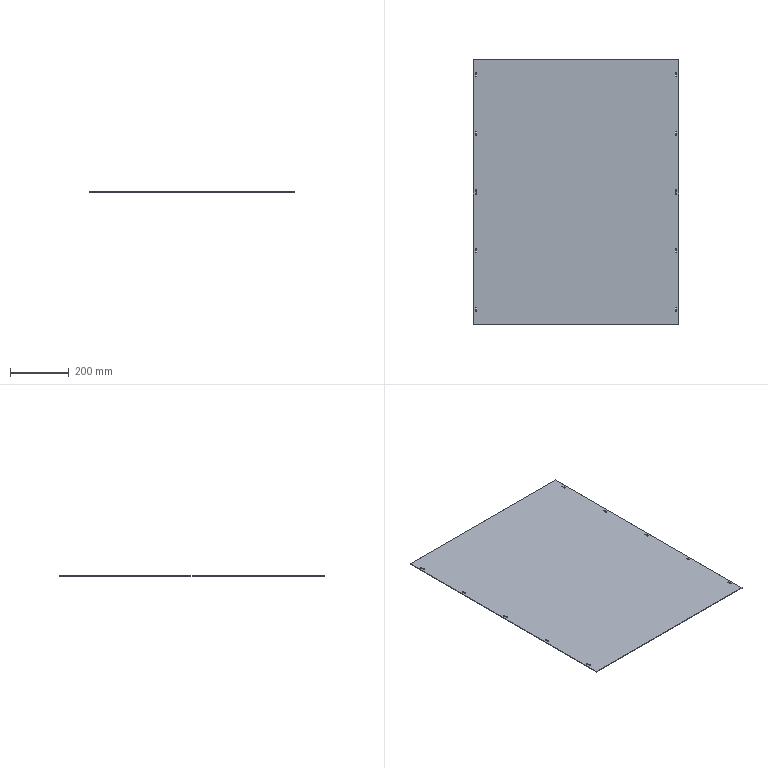Part | SolidWorks | features Extrusion 1, ICE 1 | 1 solid | 46 faces | box 700 x 900 x 2 mm | volume 1258782 mm3 | plane 26 | cylinder 20 | commonest cylinder face diameters 4.5 x20
STEP:
#1=CARTESIAN_POINT('',(350.,-450.,0.));
#2=VERTEX_POINT('',#1);
#3=CARTESIAN_POINT('',(350.,450.,0.));
#4=VERTEX_POINT('',#3);
#5=CARTESIAN_POINT('',(350.,450.,0.));
#6=DIRECTION('',(0.,1.,0.));
#7=VECTOR('',#6,1000.);
#8=LINE('',#5,#7);
#9=EDGE_CURVE('',#2,#4,#8,.T.);
#10=ORIENTED_EDGE('',*,*,#9,.T.);
#11=CARTESIAN_POINT('',(350.,450.,2.));
#12=VERTEX_POINT('',#11);
#13=CARTESIAN_POINT('',(350.,450.,2.));
#14=DIRECTION('',(0.,0.,-1.));
#15=VECTOR('',#14,1000.);
#16=LINE('',#13,#15);
#17=EDGE_CURVE('',#12,#4,#16,.T.);
#18=ORIENTED_EDGE('',*,*,#17,.F.);
#19=CARTESIAN_POINT('',(350.,-450.,2.));
#20=VERTEX_POINT('',#19);
#21=CARTESIAN_POINT('',(350.,450.,2.));
#22=DIRECTION('',(0.,1.,0.));
#23=VECTOR('',#22,1000.);
#24=LINE('',#21,#23);
#25=EDGE_CURVE('',#20,#12,#24,.T.);
#26=ORIENTED_EDGE('',*,*,#25,.F.);
#27=CARTESIAN_POINT('',(350.,-450.,2.));
#28=DIRECTION('',(0.,0.,-1.));
#29=VECTOR('',#28,1000.);
#30=LINE('',#27,#29);
#31=EDGE_CURVE('',#20,#2,#30,.T.);
#32=ORIENTED_EDGE('',*,*,#31,.T.);
#33=EDGE_LOOP('',(#10,#18,#26,#32));
#34=FACE_OUTER_BOUND('',#33,.T.);
#35=CARTESIAN_POINT('',(350.,450.,2.));
#36=DIRECTION('',(-1.,0.,0.));
#37=DIRECTION('',(0.,0.,1.));
#38=AXIS2_PLACEMENT_3D('',#35,#36,#37);
#39=PLANE('',#38);
#40=ADVANCED_FACE('',(#34),#39,.F.);
#41=CARTESIAN_POINT('',(-350.,450.,0.));
#42=VERTEX_POINT('',#41);
#43=CARTESIAN_POINT('',(-350.,450.,0.));
#44=DIRECTION('',(-1.,0.,0.));
#45=VECTOR('',#44,1000.);
#46=LINE('',#43,#45);
#47=EDGE_CURVE('',#4,#42,#46,.T.);
#48=ORIENTED_EDGE('',*,*,#47,.T.);
#49=CARTESIAN_POINT('',(-350.,450.,2.));
#50=VERTEX_POINT('',#49);
#51=CARTESIAN_POINT('',(-350.,450.,2.));
#52=DIRECTION('',(0.,0.,-1.));
#53=VECTOR('',#52,1000.);
#54=LINE('',#51,#53);
#55=EDGE_CURVE('',#50,#42,#54,.T.);
#56=ORIENTED_EDGE('',*,*,#55,.F.);
#57=CARTESIAN_POINT('',(-350.,450.,2.));
#58=DIRECTION('',(-1.,0.,0.));
#59=VECTOR('',#58,1000.);
#60=LINE('',#57,#59);
#61=EDGE_CURVE('',#12,#50,#60,.T.);
#62=ORIENTED_EDGE('',*,*,#61,.F.);
#63=ORIENTED_EDGE('',*,*,#17,.T.);
#64=EDGE_LOOP('',(#48,#56,#62,#63));
#65=FACE_OUTER_BOUND('',#64,.T.);
#66=CARTESIAN_POINT('',(-350.,450.,2.));
#67=DIRECTION('',(0.,-1.,0.));
#68=DIRECTION('',(0.,0.,-1.));
#69=AXIS2_PLACEMENT_3D('',#66,#67,#68);
#70=PLANE('',#69);
#71=ADVANCED_FACE('',(#65),#70,.F.);
#72=CARTESIAN_POINT('',(-350.,-450.,0.));
#73=VERTEX_POINT('',#72);
#74=CARTESIAN_POINT('',(-350.,450.,0.));
#75=DIRECTION('',(0.,-1.,0.));
#76=VECTOR('',#75,1000.);
#77=LINE('',#74,#76);
#78=EDGE_CURVE('',#42,#73,#77,.T.);
#79=ORIENTED_EDGE('',*,*,#78,.T.);
#80=CARTESIAN_POINT('',(-350.,-450.,2.));
#81=VERTEX_POINT('',#80);
#82=CARTESIAN_POINT('',(-350.,-450.,2.));
#83=DIRECTION('',(0.,0.,-1.));
#84=VECTOR('',#83,1000.);
#85=LINE('',#82,#84);
#86=EDGE_CURVE('',#81,#73,#85,.T.);
#87=ORIENTED_EDGE('',*,*,#86,.F.);
#88=CARTESIAN_POINT('',(-350.,450.,2.));
#89=DIRECTION('',(0.,-1.,0.));
#90=VECTOR('',#89,1000.);
#91=LINE('',#88,#90);
#92=EDGE_CURVE('',#50,#81,#91,.T.);
#93=ORIENTED_EDGE('',*,*,#92,.F.);
#94=ORIENTED_EDGE('',*,*,#55,.T.);
#95=EDGE_LOOP('',(#79,#87,#93,#94));
#96=FACE_OUTER_BOUND('',#95,.T.);
#97=CARTESIAN_POINT('',(-350.,450.,2.));
#98=DIRECTION('',(1.,0.,0.));
#99=DIRECTION('',(0.,0.,-1.));
#100=AXIS2_PLACEMENT_3D('',#97,#98,#99);
#101=PLANE('',#100);
#102=ADVANCED_FACE('',(#96),#101,.F.);
#103=CARTESIAN_POINT('',(-350.,-450.,0.));
#104=DIRECTION('',(1.,0.,0.));
#105=VECTOR('',#104,1000.);
#106=LINE('',#103,#105);
#107=EDGE_CURVE('',#73,#2,#106,.T.);
#108=ORIENTED_EDGE('',*,*,#107,.T.);
#109=ORIENTED_EDGE('',*,*,#31,.F.);
#110=CARTESIAN_POINT('',(-350.,-450.,2.));
#111=DIRECTION('',(1.,0.,0.));
#112=VECTOR('',#111,1000.);
#113=LINE('',#110,#112);
#114=EDGE_CURVE('',#81,#20,#113,.T.);
#115=ORIENTED_EDGE('',*,*,#114,.F.);
#116=ORIENTED_EDGE('',*,*,#86,.T.);
#117=EDGE_LOOP('',(#108,#109,#115,#116));
#118=FACE_OUTER_BOUND('',#117,.T.);
#119=CARTESIAN_POINT('',(-350.,-450.,2.));
#120=DIRECTION('',(0.,1.,0.));
#121=DIRECTION('',(0.,0.,1.));
#122=AXIS2_PLACEMENT_3D('',#119,#120,#121);
#123=PLANE('',#122);
#124=ADVANCED_FACE('',(#118),#123,.F.);
#125=CARTESIAN_POINT('',(337.75,-5.,2.));
#126=VERTEX_POINT('',#125);
#127=CARTESIAN_POINT('',(342.25,-5.,2.));
#128=VERTEX_POINT('',#127);
#129=CARTESIAN_POINT('',(340.,-5.,2.));
#130=DIRECTION('',(0.,0.,1.));
#131=DIRECTION('',(-1.,0.,0.));
#132=AXIS2_PLACEMENT_3D('',#129,#130,#131);
#133=CIRCLE('',#132,2.25);
#134=EDGE_CURVE('',#126,#128,#133,.T.);
#135=ORIENTED_EDGE('',*,*,#134,.F.);
#136=CARTESIAN_POINT('',(337.75,5.,2.));
#137=VERTEX_POINT('',#136);
#138=CARTESIAN_POINT('',(337.75,-5.,2.));
#139=DIRECTION('',(0.,-1.,0.));
#140=VECTOR('',#139,1000.);
#141=LINE('',#138,#140);
#142=EDGE_CURVE('',#137,#126,#141,.T.);
#143=ORIENTED_EDGE('',*,*,#142,.F.);
#144=CARTESIAN_POINT('',(342.25,5.,2.));
#145=VERTEX_POINT('',#144);
#146=CARTESIAN_POINT('',(340.,5.,2.));
#147=DIRECTION('',(0.,0.,1.));
#148=DIRECTION('',(-1.,0.,0.));
#149=AXIS2_PLACEMENT_3D('',#146,#147,#148);
#150=CIRCLE('',#149,2.25);
#151=EDGE_CURVE('',#145,#137,#150,.T.);
#152=ORIENTED_EDGE('',*,*,#151,.F.);
#153=CARTESIAN_POINT('',(342.25,-5.,2.));
#154=DIRECTION('',(0.,1.,0.));
#155=VECTOR('',#154,1000.);
#156=LINE('',#153,#155);
#157=EDGE_CURVE('',#128,#145,#156,.T.);
#158=ORIENTED_EDGE('',*,*,#157,.F.);
#159=EDGE_LOOP('',(#135,#143,#152,#158));
#160=FACE_BOUND('',#159,.T.);
#161=CARTESIAN_POINT('',(342.25,-195.,2.));
#162=VERTEX_POINT('',#161);
#163=CARTESIAN_POINT('',(337.75,-195.,2.));
#164=VERTEX_POINT('',#163);
#165=CARTESIAN_POINT('',(340.,-195.,2.));
#166=DIRECTION('',(0.,0.,1.));
#167=DIRECTION('',(1.,0.,0.));
#168=AXIS2_PLACEMENT_3D('',#165,#166,#167);
#169=CIRCLE('',#168,2.25);
#170=EDGE_CURVE('',#162,#164,#169,.T.);
#171=ORIENTED_EDGE('',*,*,#170,.F.);
#172=CARTESIAN_POINT('',(342.25,-205.,2.));
#173=VERTEX_POINT('',#172);
#174=CARTESIAN_POINT('',(342.25,-195.,2.));
#175=DIRECTION('',(0.,1.,0.));
#176=VECTOR('',#175,1000.);
#177=LINE('',#174,#176);
#178=EDGE_CURVE('',#173,#162,#177,.T.);
#179=ORIENTED_EDGE('',*,*,#178,.F.);
#180=CARTESIAN_POINT('',(337.75,-205.,2.));
#181=VERTEX_POINT('',#180);
#182=CARTESIAN_POINT('',(340.,-205.,2.));
#183=DIRECTION('',(0.,0.,1.));
#184=DIRECTION('',(1.,0.,0.));
#185=AXIS2_PLACEMENT_3D('',#182,#183,#184);
#186=CIRCLE('',#185,2.25);
#187=EDGE_CURVE('',#181,#173,#186,.T.);
#188=ORIENTED_EDGE('',*,*,#187,.F.);
#189=CARTESIAN_POINT('',(337.75,-195.,2.));
#190=DIRECTION('',(0.,-1.,0.));
#191=VECTOR('',#190,1000.);
#192=LINE('',#189,#191);
#193=EDGE_CURVE('',#164,#181,#192,.T.);
#194=ORIENTED_EDGE('',*,*,#193,.F.);
#195=EDGE_LOOP('',(#171,#179,#188,#194));
#196=FACE_BOUND('',#195,.T.);
#197=CARTESIAN_POINT('',(342.25,405.,2.));
#198=VERTEX_POINT('',#197);
#199=CARTESIAN_POINT('',(337.75,405.,2.));
#200=VERTEX_POINT('',#199);
#201=CARTESIAN_POINT('',(340.,405.,2.));
#202=DIRECTION('',(0.,0.,1.));
#203=DIRECTION('',(-1.,0.,0.));
#204=AXIS2_PLACEMENT_3D('',#201,#202,#203);
#205=CIRCLE('',#204,2.25);
#206=EDGE_CURVE('',#198,#200,#205,.T.);
#207=ORIENTED_EDGE('',*,*,#206,.F.);
#208=CARTESIAN_POINT('',(342.25,395.,2.));
#209=VERTEX_POINT('',#208);
#210=CARTESIAN_POINT('',(342.25,405.,2.));
#211=DIRECTION('',(0.,1.,0.));
#212=VECTOR('',#211,1000.);
#213=LINE('',#210,#212);
#214=EDGE_CURVE('',#209,#198,#213,.T.);
#215=ORIENTED_EDGE('',*,*,#214,.F.);
#216=CARTESIAN_POINT('',(337.75,395.,2.));
#217=VERTEX_POINT('',#216);
#218=CARTESIAN_POINT('',(340.,395.,2.));
#219=DIRECTION('',(0.,0.,1.));
#220=DIRECTION('',(-1.,0.,0.));
#221=AXIS2_PLACEMENT_3D('',#218,#219,#220);
#222=CIRCLE('',#221,2.25);
#223=EDGE_CURVE('',#217,#209,#222,.T.);
#224=ORIENTED_EDGE('',*,*,#223,.F.);
#225=CARTESIAN_POINT('',(337.75,405.,2.));
#226=DIRECTION('',(0.,-1.,0.));
#227=VECTOR('',#226,1000.);
#228=LINE('',#225,#227);
#229=EDGE_CURVE('',#200,#217,#228,.T.);
#230=ORIENTED_EDGE('',*,*,#229,.F.);
#231=EDGE_LOOP('',(#207,#215,#224,#230));
#232=FACE_BOUND('',#231,.T.);
#233=CARTESIAN_POINT('',(-342.25,195.,2.));
#234=VERTEX_POINT('',#233);
#235=CARTESIAN_POINT('',(-337.75,195.,2.));
#236=VERTEX_POINT('',#235);
#237=CARTESIAN_POINT('',(-340.,195.,2.));
#238=DIRECTION('',(0.,0.,1.));
#239=DIRECTION('',(1.,0.,0.));
#240=AXIS2_PLACEMENT_3D('',#237,#238,#239);
#241=CIRCLE('',#240,2.25);
#242=EDGE_CURVE('',#234,#236,#241,.T.);
#243=ORIENTED_EDGE('',*,*,#242,.F.);
#244=CARTESIAN_POINT('',(-342.25,205.,2.));
#245=VERTEX_POINT('',#244);
#246=CARTESIAN_POINT('',(-342.25,195.,2.));
#247=DIRECTION('',(0.,-1.,0.));
#248=VECTOR('',#247,1000.);
#249=LINE('',#246,#248);
#250=EDGE_CURVE('',#245,#234,#249,.T.);
#251=ORIENTED_EDGE('',*,*,#250,.F.);
#252=CARTESIAN_POINT('',(-337.75,205.,2.));
#253=VERTEX_POINT('',#252);
#254=CARTESIAN_POINT('',(-340.,205.,2.));
#255=DIRECTION('',(0.,0.,1.));
#256=DIRECTION('',(1.,0.,0.));
#257=AXIS2_PLACEMENT_3D('',#254,#255,#256);
#258=CIRCLE('',#257,2.25);
#259=EDGE_CURVE('',#253,#245,#258,.T.);
#260=ORIENTED_EDGE('',*,*,#259,.F.);
#261=CARTESIAN_POINT('',(-337.75,195.,2.));
#262=DIRECTION('',(0.,1.,0.));
#263=VECTOR('',#262,1000.);
#264=LINE('',#261,#263);
#265=EDGE_CURVE('',#236,#253,#264,.T.);
#266=ORIENTED_EDGE('',*,*,#265,.F.);
#267=EDGE_LOOP('',(#243,#251,#260,#266));
#268=FACE_BOUND('',#267,.T.);
#269=CARTESIAN_POINT('',(-342.25,-5.,2.));
#270=VERTEX_POINT('',#269);
#271=CARTESIAN_POINT('',(-337.75,-5.,2.));
#272=VERTEX_POINT('',#271);
#273=CARTESIAN_POINT('',(-340.,-5.,2.));
#274=DIRECTION('',(0.,0.,1.));
#275=DIRECTION('',(1.,0.,0.));
#276=AXIS2_PLACEMENT_3D('',#273,#274,#275);
#277=CIRCLE('',#276,2.25);
#278=EDGE_CURVE('',#270,#272,#277,.T.);
#279=ORIENTED_EDGE('',*,*,#278,.F.);
#280=CARTESIAN_POINT('',(-342.25,5.,2.));
#281=VERTEX_POINT('',#280);
#282=CARTESIAN_POINT('',(-342.25,-5.,2.));
#283=DIRECTION('',(0.,-1.,0.));
#284=VECTOR('',#283,1000.);
#285=LINE('',#282,#284);
#286=EDGE_CURVE('',#281,#270,#285,.T.);
#287=ORIENTED_EDGE('',*,*,#286,.F.);
#288=CARTESIAN_POINT('',(-337.75,5.,2.));
#289=VERTEX_POINT('',#288);
#290=CARTESIAN_POINT('',(-340.,5.,2.));
#291=DIRECTION('',(0.,0.,1.));
#292=DIRECTION('',(1.,0.,0.));
#293=AXIS2_PLACEMENT_3D('',#290,#291,#292);
#294=CIRCLE('',#293,2.25);
#295=EDGE_CURVE('',#289,#281,#294,.T.);
#296=ORIENTED_EDGE('',*,*,#295,.F.);
#297=CARTESIAN_POINT('',(-337.75,-5.,2.));
#298=DIRECTION('',(0.,1.,0.));
#299=VECTOR('',#298,1000.);
#300=LINE('',#297,#299);
#301=EDGE_CURVE('',#272,#289,#300,.T.);
#302=ORIENTED_EDGE('',*,*,#301,.F.);
#303=EDGE_LOOP('',(#279,#287,#296,#302));
#304=FACE_BOUND('',#303,.T.);
#305=CARTESIAN_POINT('',(337.75,195.,2.));
#306=VERTEX_POINT('',#305);
#307=CARTESIAN_POINT('',(342.25,195.,2.));
#308=VERTEX_POINT('',#307);
#309=CARTESIAN_POINT('',(340.,195.,2.));
#310=DIRECTION('',(0.,0.,1.));
#311=DIRECTION('',(-1.,0.,0.));
#312=AXIS2_PLACEMENT_3D('',#309,#310,#311);
#313=CIRCLE('',#312,2.25);
#314=EDGE_CURVE('',#306,#308,#313,.T.);
#315=ORIENTED_EDGE('',*,*,#314,.F.);
#316=CARTESIAN_POINT('',(337.75,205.,2.));
#317=VERTEX_POINT('',#316);
#318=CARTESIAN_POINT('',(337.75,195.,2.));
#319=DIRECTION('',(0.,-1.,0.));
#320=VECTOR('',#319,1000.);
#321=LINE('',#318,#320);
#322=EDGE_CURVE('',#317,#306,#321,.T.);
#323=ORIENTED_EDGE('',*,*,#322,.F.);
#324=CARTESIAN_POINT('',(342.25,205.,2.));
#325=VERTEX_POINT('',#324);
#326=CARTESIAN_POINT('',(340.,205.,2.));
#327=DIRECTION('',(0.,0.,1.));
#328=DIRECTION('',(-1.,0.,0.));
#329=AXIS2_PLACEMENT_3D('',#326,#327,#328);
#330=CIRCLE('',#329,2.25);
#331=EDGE_CURVE('',#325,#317,#330,.T.);
#332=ORIENTED_EDGE('',*,*,#331,.F.);
#333=CARTESIAN_POINT('',(342.25,195.,2.));
#334=DIRECTION('',(0.,1.,0.));
#335=VECTOR('',#334,1000.);
#336=LINE('',#333,#335);
#337=EDGE_CURVE('',#308,#325,#336,.T.);
#338=ORIENTED_EDGE('',*,*,#337,.F.);
#339=EDGE_LOOP('',(#315,#323,#332,#338));
#340=FACE_BOUND('',#339,.T.);
#341=CARTESIAN_POINT('',(-342.25,-405.,2.));
#342=VERTEX_POINT('',#341);
#343=CARTESIAN_POINT('',(-337.75,-405.,2.));
#344=VERTEX_POINT('',#343);
#345=CARTESIAN_POINT('',(-340.,-405.,2.));
#346=DIRECTION('',(0.,0.,1.));
#347=DIRECTION('',(-1.,0.,0.));
#348=AXIS2_PLACEMENT_3D('',#345,#346,#347);
#349=CIRCLE('',#348,2.25);
#350=EDGE_CURVE('',#342,#344,#349,.T.);
#351=ORIENTED_EDGE('',*,*,#350,.F.);
#352=CARTESIAN_POINT('',(-342.25,-395.,2.));
#353=VERTEX_POINT('',#352);
#354=CARTESIAN_POINT('',(-342.25,-405.,2.));
#355=DIRECTION('',(0.,-1.,0.));
#356=VECTOR('',#355,1000.);
#357=LINE('',#354,#356);
#358=EDGE_CURVE('',#353,#342,#357,.T.);
#359=ORIENTED_EDGE('',*,*,#358,.F.);
#360=CARTESIAN_POINT('',(-337.75,-395.,2.));
#361=VERTEX_POINT('',#360);
#362=CARTESIAN_POINT('',(-340.,-395.,2.));
#363=DIRECTION('',(0.,0.,1.));
#364=DIRECTION('',(-1.,0.,0.));
#365=AXIS2_PLACEMENT_3D('',#362,#363,#364);
#366=CIRCLE('',#365,2.25);
#367=EDGE_CURVE('',#361,#353,#366,.T.);
#368=ORIENTED_EDGE('',*,*,#367,.F.);
#369=CARTESIAN_POINT('',(-337.75,-405.,2.));
#370=DIRECTION('',(0.,1.,0.));
#371=VECTOR('',#370,1000.);
#372=LINE('',#369,#371);
#373=EDGE_CURVE('',#344,#361,#372,.T.);
#374=ORIENTED_EDGE('',*,*,#373,.F.);
#375=EDGE_LOOP('',(#351,#359,#368,#374));
#376=FACE_BOUND('',#375,.T.);
#377=CARTESIAN_POINT('',(337.75,-405.,2.));
#378=VERTEX_POINT('',#377);
#379=CARTESIAN_POINT('',(342.25,-405.,2.));
#380=VERTEX_POINT('',#379);
#381=CARTESIAN_POINT('',(340.,-405.,2.));
#382=DIRECTION('',(0.,0.,1.));
#383=DIRECTION('',(1.,0.,0.));
#384=AXIS2_PLACEMENT_3D('',#381,#382,#383);
#385=CIRCLE('',#384,2.25);
#386=EDGE_CURVE('',#378,#380,#385,.T.);
#387=ORIENTED_EDGE('',*,*,#386,.F.);
#388=CARTESIAN_POINT('',(337.75,-395.,2.));
#389=VERTEX_POINT('',#388);
#390=CARTESIAN_POINT('',(337.75,-405.,2.));
#391=DIRECTION('',(0.,-1.,0.));
#392=VECTOR('',#391,1000.);
#393=LINE('',#390,#392);
#394=EDGE_CURVE('',#389,#378,#393,.T.);
#395=ORIENTED_EDGE('',*,*,#394,.F.);
#396=CARTESIAN_POINT('',(342.25,-395.,2.));
#397=VERTEX_POINT('',#396);
#398=CARTESIAN_POINT('',(340.,-395.,2.));
#399=DIRECTION('',(0.,0.,1.));
#400=DIRECTION('',(1.,0.,0.));
#401=AXIS2_PLACEMENT_3D('',#398,#399,#400);
#402=CIRCLE('',#401,2.25);
#403=EDGE_CURVE('',#397,#389,#402,.T.);
#404=ORIENTED_EDGE('',*,*,#403,.F.);
#405=CARTESIAN_POINT('',(342.25,-405.,2.));
#406=DIRECTION('',(0.,1.,0.));
#407=VECTOR('',#406,1000.);
#408=LINE('',#405,#407);
#409=EDGE_CURVE('',#380,#397,#408,.T.);
#410=ORIENTED_EDGE('',*,*,#409,.F.);
#411=EDGE_LOOP('',(#387,#395,#404,#410));
#412=FACE_BOUND('',#411,.T.);
#413=CARTESIAN_POINT('',(-337.75,-195.,2.));
#414=VERTEX_POINT('',#413);
#415=CARTESIAN_POINT('',(-342.25,-195.,2.));
#416=VERTEX_POINT('',#415);
#417=CARTESIAN_POINT('',(-340.,-195.,2.));
#418=DIRECTION('',(0.,0.,1.));
#419=DIRECTION('',(-1.,0.,0.));
#420=AXIS2_PLACEMENT_3D('',#417,#418,#419);
#421=CIRCLE('',#420,2.25);
#422=EDGE_CURVE('',#414,#416,#421,.T.);
#423=ORIENTED_EDGE('',*,*,#422,.F.);
#424=CARTESIAN_POINT('',(-337.75,-205.,2.));
#425=VERTEX_POINT('',#424);
#426=CARTESIAN_POINT('',(-337.75,-195.,2.));
#427=DIRECTION('',(0.,1.,0.));
#428=VECTOR('',#427,1000.);
#429=LINE('',#426,#428);
#430=EDGE_CURVE('',#425,#414,#429,.T.);
#431=ORIENTED_EDGE('',*,*,#430,.F.);
#432=CARTESIAN_POINT('',(-342.25,-205.,2.));
#433=VERTEX_POINT('',#432);
#434=CARTESIAN_POINT('',(-340.,-205.,2.));
#435=DIRECTION('',(0.,0.,1.));
#436=DIRECTION('',(-1.,0.,0.));
#437=AXIS2_PLACEMENT_3D('',#434,#435,#436);
#438=CIRCLE('',#437,2.25);
#439=EDGE_CURVE('',#433,#425,#438,.T.);
#440=ORIENTED_EDGE('',*,*,#439,.F.);
#441=CARTESIAN_POINT('',(-342.25,-195.,2.));
#442=DIRECTION('',(0.,-1.,0.));
#443=VECTOR('',#442,1000.);
#444=LINE('',#441,#443);
#445=EDGE_CURVE('',#416,#433,#444,.T.);
#446=ORIENTED_EDGE('',*,*,#445,.F.);
#447=EDGE_LOOP('',(#423,#431,#440,#446));
#448=FACE_BOUND('',#447,.T.);
#449=CARTESIAN_POINT('',(-337.75,405.,2.));
#450=VERTEX_POINT('',#449);
#451=CARTESIAN_POINT('',(-342.25,405.,2.));
#452=VERTEX_POINT('',#451);
#453=CARTESIAN_POINT('',(-340.,405.,2.));
#454=DIRECTION('',(0.,0.,1.));
#455=DIRECTION('',(1.,0.,0.));
#456=AXIS2_PLACEMENT_3D('',#453,#454,#455);
#457=CIRCLE('',#456,2.25);
#458=EDGE_CURVE('',#450,#452,#457,.T.);
#459=ORIENTED_EDGE('',*,*,#458,.F.);
#460=CARTESIAN_POINT('',(-337.75,395.,2.));
#461=VERTEX_POINT('',#460);
#462=CARTESIAN_POINT('',(-337.75,405.,2.));
#463=DIRECTION('',(0.,1.,0.));
#464=VECTOR('',#463,1000.);
#465=LINE('',#462,#464);
#466=EDGE_CURVE('',#461,#450,#465,.T.);
#467=ORIENTED_EDGE('',*,*,#466,.F.);
#468=CARTESIAN_POINT('',(-342.25,395.,2.));
#469=VERTEX_POINT('',#468);
#470=CARTESIAN_POINT('',(-340.,395.,2.));
#471=DIRECTION('',(0.,0.,1.));
#472=DIRECTION('',(1.,0.,0.));
#473=AXIS2_PLACEMENT_3D('',#470,#471,#472);
#474=CIRCLE('',#473,2.25);
#475=EDGE_CURVE('',#469,#461,#474,.T.);
#476=ORIENTED_EDGE('',*,*,#475,.F.);
#477=CARTESIAN_POINT('',(-342.25,405.,2.));
#478=DIRECTION('',(0.,-1.,0.));
#479=VECTOR('',#478,1000.);
#480=LINE('',#477,#479);
#481=EDGE_CURVE('',#452,#469,#480,.T.);
#482=ORIENTED_EDGE('',*,*,#481,.F.);
#483=EDGE_LOOP('',(#459,#467,#476,#482));
#484=FACE_BOUND('',#483,.T.);
#485=ORIENTED_EDGE('',*,*,#25,.T.);
#486=ORIENTED_EDGE('',*,*,#61,.T.);
#487=ORIENTED_EDGE('',*,*,#92,.T.);
#488=ORIENTED_EDGE('',*,*,#114,.T.);
#489=EDGE_LOOP('',(#485,#486,#487,#488));
#490=FACE_OUTER_BOUND('',#489,.T.);
#491=CARTESIAN_POINT('',(0.,0.,2.));
#492=DIRECTION('',(0.,0.,1.));
#493=DIRECTION('',(1.,0.,0.));
#494=AXIS2_PLACEMENT_3D('',#491,#492,#493);
#495=PLANE('',#494);
#496=ADVANCED_FACE('',(#160,#196,#232,#268,#304,#340,#376,#412,#448,#484,#490),#495,.T.);
#497=CARTESIAN_POINT('',(337.75,5.,0.));
#498=VERTEX_POINT('',#497);
#499=CARTESIAN_POINT('',(337.75,-5.,0.));
#500=VERTEX_POINT('',#499);
#501=CARTESIAN_POINT('',(337.75,0.,0.));
#502=DIRECTION('',(0.,-1.,0.));
#503=VECTOR('',#502,1000.);
#504=LINE('',#501,#503);
#505=EDGE_CURVE('',#498,#500,#504,.T.);
#506=ORIENTED_EDGE('',*,*,#505,.T.);
#507=CARTESIAN_POINT('',(342.25,-5.,0.));
#508=VERTEX_POINT('',#507);
#509=CARTESIAN_POINT('',(340.,-5.,0.));
#510=DIRECTION('',(0.,0.,1.));
#511=DIRECTION('',(1.,0.,0.));
#512=AXIS2_PLACEMENT_3D('',#509,#510,#511);
#513=CIRCLE('',#512,2.25);
#514=EDGE_CURVE('',#500,#508,#513,.T.);
#515=ORIENTED_EDGE('',*,*,#514,.T.);
#516=CARTESIAN_POINT('',(342.25,5.,0.));
#517=VERTEX_POINT('',#516);
#518=CARTESIAN_POINT('',(342.25,0.,0.));
#519=DIRECTION('',(0.,1.,0.));
#520=VECTOR('',#519,1000.);
#521=LINE('',#518,#520);
#522=EDGE_CURVE('',#508,#517,#521,.T.);
#523=ORIENTED_EDGE('',*,*,#522,.T.);
#524=CARTESIAN_POINT('',(340.,5.,0.));
#525=DIRECTION('',(0.,0.,1.));
#526=DIRECTION('',(1.,0.,0.));
#527=AXIS2_PLACEMENT_3D('',#524,#525,#526);
#528=CIRCLE('',#527,2.25);
#529=EDGE_CURVE('',#517,#498,#528,.T.);
#530=ORIENTED_EDGE('',*,*,#529,.T.);
#531=EDGE_LOOP('',(#506,#515,#523,#530));
#532=FACE_BOUND('',#531,.T.);
#533=CARTESIAN_POINT('',(342.25,-205.,0.));
#534=VERTEX_POINT('',#533);
#535=CARTESIAN_POINT('',(342.25,-195.,0.));
#536=VERTEX_POINT('',#535);
#537=CARTESIAN_POINT('',(342.25,0.,0.));
#538=DIRECTION('',(0.,1.,0.));
#539=VECTOR('',#538,1000.);
#540=LINE('',#537,#539);
#541=EDGE_CURVE('',#534,#536,#540,.T.);
#542=ORIENTED_EDGE('',*,*,#541,.T.);
#543=CARTESIAN_POINT('',(337.75,-195.,0.));
#544=VERTEX_POINT('',#543);
#545=CARTESIAN_POINT('',(340.,-195.,0.));
#546=DIRECTION('',(0.,0.,1.));
#547=DIRECTION('',(1.,0.,0.));
#548=AXIS2_PLACEMENT_3D('',#545,#546,#547);
#549=CIRCLE('',#548,2.25);
#550=EDGE_CURVE('',#536,#544,#549,.T.);
#551=ORIENTED_EDGE('',*,*,#550,.T.);
#552=CARTESIAN_POINT('',(337.75,-205.,0.));
#553=VERTEX_POINT('',#552);
#554=CARTESIAN_POINT('',(337.75,0.,0.));
#555=DIRECTION('',(0.,-1.,0.));
#556=VECTOR('',#555,1000.);
#557=LINE('',#554,#556);
#558=EDGE_CURVE('',#544,#553,#557,.T.);
#559=ORIENTED_EDGE('',*,*,#558,.T.);
#560=CARTESIAN_POINT('',(340.,-205.,0.));
#561=DIRECTION('',(0.,0.,1.));
#562=DIRECTION('',(1.,0.,0.));
#563=AXIS2_PLACEMENT_3D('',#560,#561,#562);
#564=CIRCLE('',#563,2.25);
#565=EDGE_CURVE('',#553,#534,#564,.T.);
#566=ORIENTED_EDGE('',*,*,#565,.T.);
#567=EDGE_LOOP('',(#542,#551,#559,#566));
#568=FACE_BOUND('',#567,.T.);
#569=CARTESIAN_POINT('',(342.25,395.,0.));
#570=VERTEX_POINT('',#569);
#571=CARTESIAN_POINT('',(342.25,405.,0.));
#572=VERTEX_POINT('',#571);
#573=CARTESIAN_POINT('',(342.25,0.,0.));
#574=DIRECTION('',(0.,1.,0.));
#575=VECTOR('',#574,1000.);
#576=LINE('',#573,#575);
#577=EDGE_CURVE('',#570,#572,#576,.T.);
#578=ORIENTED_EDGE('',*,*,#577,.T.);
#579=CARTESIAN_POINT('',(337.75,405.,0.));
#580=VERTEX_POINT('',#579);
#581=CARTESIAN_POINT('',(340.,405.,0.));
#582=DIRECTION('',(0.,0.,1.));
#583=DIRECTION('',(1.,0.,0.));
#584=AXIS2_PLACEMENT_3D('',#581,#582,#583);
#585=CIRCLE('',#584,2.25);
#586=EDGE_CURVE('',#572,#580,#585,.T.);
#587=ORIENTED_EDGE('',*,*,#586,.T.);
#588=CARTESIAN_POINT('',(337.75,395.,0.));
#589=VERTEX_POINT('',#588);
#590=CARTESIAN_POINT('',(337.75,0.,0.));
#591=DIRECTION('',(0.,-1.,0.));
#592=VECTOR('',#591,1000.);
#593=LINE('',#590,#592);
#594=EDGE_CURVE('',#580,#589,#593,.T.);
#595=ORIENTED_EDGE('',*,*,#594,.T.);
#596=CARTESIAN_POINT('',(340.,395.,0.));
#597=DIRECTION('',(0.,0.,1.));
#598=DIRECTION('',(1.,0.,0.));
#599=AXIS2_PLACEMENT_3D('',#596,#597,#598);
#600=CIRCLE('',#599,2.25);
#601=EDGE_CURVE('',#589,#570,#600,.T.);
#602=ORIENTED_EDGE('',*,*,#601,.T.);
#603=EDGE_LOOP('',(#578,#587,#595,#602));
#604=FACE_BOUND('',#603,.T.);
#605=CARTESIAN_POINT('',(-342.25,205.,0.));
#606=VERTEX_POINT('',#605);
#607=CARTESIAN_POINT('',(-342.25,195.,0.));
#608=VERTEX_POINT('',#607);
#609=CARTESIAN_POINT('',(-342.25,0.,0.));
#610=DIRECTION('',(0.,-1.,0.));
#611=VECTOR('',#610,1000.);
#612=LINE('',#609,#611);
#613=EDGE_CURVE('',#606,#608,#612,.T.);
#614=ORIENTED_EDGE('',*,*,#613,.T.);
#615=CARTESIAN_POINT('',(-337.75,195.,0.));
#616=VERTEX_POINT('',#615);
#617=CARTESIAN_POINT('',(-340.,195.,0.));
#618=DIRECTION('',(0.,0.,1.));
#619=DIRECTION('',(1.,0.,0.));
#620=AXIS2_PLACEMENT_3D('',#617,#618,#619);
#621=CIRCLE('',#620,2.25);
#622=EDGE_CURVE('',#608,#616,#621,.T.);
#623=ORIENTED_EDGE('',*,*,#622,.T.);
#624=CARTESIAN_POINT('',(-337.75,205.,0.));
#625=VERTEX_POINT('',#624);
#626=CARTESIAN_POINT('',(-337.75,0.,0.));
#627=DIRECTION('',(0.,1.,0.));
#628=VECTOR('',#627,1000.);
#629=LINE('',#626,#628);
#630=EDGE_CURVE('',#616,#625,#629,.T.);
#631=ORIENTED_EDGE('',*,*,#630,.T.);
#632=CARTESIAN_POINT('',(-340.,205.,0.));
#633=DIRECTION('',(0.,0.,1.));
#634=DIRECTION('',(1.,0.,0.));
#635=AXIS2_PLACEMENT_3D('',#632,#633,#634);
#636=CIRCLE('',#635,2.25);
#637=EDGE_CURVE('',#625,#606,#636,.T.);
#638=ORIENTED_EDGE('',*,*,#637,.T.);
#639=EDGE_LOOP('',(#614,#623,#631,#638));
#640=FACE_BOUND('',#639,.T.);
#641=CARTESIAN_POINT('',(-342.25,5.,0.));
#642=VERTEX_POINT('',#641);
#643=CARTESIAN_POINT('',(-342.25,-5.,0.));
#644=VERTEX_POINT('',#643);
#645=CARTESIAN_POINT('',(-342.25,0.,0.));
#646=DIRECTION('',(0.,-1.,0.));
#647=VECTOR('',#646,1000.);
#648=LINE('',#645,#647);
#649=EDGE_CURVE('',#642,#644,#648,.T.);
#650=ORIENTED_EDGE('',*,*,#649,.T.);
#651=CARTESIAN_POINT('',(-337.75,-5.,0.));
#652=VERTEX_POINT('',#651);
#653=CARTESIAN_POINT('',(-340.,-5.,0.));
#654=DIRECTION('',(0.,0.,1.));
#655=DIRECTION('',(1.,0.,0.));
#656=AXIS2_PLACEMENT_3D('',#653,#654,#655);
#657=CIRCLE('',#656,2.25);
#658=EDGE_CURVE('',#644,#652,#657,.T.);
#659=ORIENTED_EDGE('',*,*,#658,.T.);
#660=CARTESIAN_POINT('',(-337.75,5.,0.));
#661=VERTEX_POINT('',#660);
#662=CARTESIAN_POINT('',(-337.75,0.,0.));
#663=DIRECTION('',(0.,1.,0.));
#664=VECTOR('',#663,1000.);
#665=LINE('',#662,#664);
#666=EDGE_CURVE('',#652,#661,#665,.T.);
#667=ORIENTED_EDGE('',*,*,#666,.T.);
#668=CARTESIAN_POINT('',(-340.,5.,0.));
#669=DIRECTION('',(0.,0.,1.));
#670=DIRECTION('',(1.,0.,0.));
#671=AXIS2_PLACEMENT_3D('',#668,#669,#670);
#672=CIRCLE('',#671,2.25);
#673=EDGE_CURVE('',#661,#642,#672,.T.);
#674=ORIENTED_EDGE('',*,*,#673,.T.);
#675=EDGE_LOOP('',(#650,#659,#667,#674));
#676=FACE_BOUND('',#675,.T.);
#677=CARTESIAN_POINT('',(337.75,205.,0.));
#678=VERTEX_POINT('',#677);
#679=CARTESIAN_POINT('',(337.75,195.,0.));
#680=VERTEX_POINT('',#679);
#681=CARTESIAN_POINT('',(337.75,0.,0.));
#682=DIRECTION('',(0.,-1.,0.));
#683=VECTOR('',#682,1000.);
#684=LINE('',#681,#683);
#685=EDGE_CURVE('',#678,#680,#684,.T.);
#686=ORIENTED_EDGE('',*,*,#685,.T.);
#687=CARTESIAN_POINT('',(342.25,195.,0.));
#688=VERTEX_POINT('',#687);
#689=CARTESIAN_POINT('',(340.,195.,0.));
#690=DIRECTION('',(0.,0.,1.));
#691=DIRECTION('',(1.,0.,0.));
#692=AXIS2_PLACEMENT_3D('',#689,#690,#691);
#693=CIRCLE('',#692,2.25);
#694=EDGE_CURVE('',#680,#688,#693,.T.);
#695=ORIENTED_EDGE('',*,*,#694,.T.);
#696=CARTESIAN_POINT('',(342.25,205.,0.));
#697=VERTEX_POINT('',#696);
#698=CARTESIAN_POINT('',(342.25,0.,0.));
#699=DIRECTION('',(0.,1.,0.));
#700=VECTOR('',#699,1000.);
#701=LINE('',#698,#700);
#702=EDGE_CURVE('',#688,#697,#701,.T.);
#703=ORIENTED_EDGE('',*,*,#702,.T.);
#704=CARTESIAN_POINT('',(340.,205.,0.));
#705=DIRECTION('',(0.,0.,1.));
#706=DIRECTION('',(1.,0.,0.));
#707=AXIS2_PLACEMENT_3D('',#704,#705,#706);
#708=CIRCLE('',#707,2.25);
#709=EDGE_CURVE('',#697,#678,#708,.T.);
#710=ORIENTED_EDGE('',*,*,#709,.T.);
#711=EDGE_LOOP('',(#686,#695,#703,#710));
#712=FACE_BOUND('',#711,.T.);
#713=CARTESIAN_POINT('',(-342.25,-395.,0.));
#714=VERTEX_POINT('',#713);
#715=CARTESIAN_POINT('',(-342.25,-405.,0.));
#716=VERTEX_POINT('',#715);
#717=CARTESIAN_POINT('',(-342.25,0.,0.));
#718=DIRECTION('',(0.,-1.,0.));
#719=VECTOR('',#718,1000.);
#720=LINE('',#717,#719);
#721=EDGE_CURVE('',#714,#716,#720,.T.);
#722=ORIENTED_EDGE('',*,*,#721,.T.);
#723=CARTESIAN_POINT('',(-337.75,-405.,0.));
#724=VERTEX_POINT('',#723);
#725=CARTESIAN_POINT('',(-340.,-405.,0.));
#726=DIRECTION('',(0.,0.,1.));
#727=DIRECTION('',(1.,0.,0.));
#728=AXIS2_PLACEMENT_3D('',#725,#726,#727);
#729=CIRCLE('',#728,2.25);
#730=EDGE_CURVE('',#716,#724,#729,.T.);
#731=ORIENTED_EDGE('',*,*,#730,.T.);
#732=CARTESIAN_POINT('',(-337.75,-395.,0.));
#733=VERTEX_POINT('',#732);
#734=CARTESIAN_POINT('',(-337.75,0.,0.));
#735=DIRECTION('',(0.,1.,0.));
#736=VECTOR('',#735,1000.);
#737=LINE('',#734,#736);
#738=EDGE_CURVE('',#724,#733,#737,.T.);
#739=ORIENTED_EDGE('',*,*,#738,.T.);
#740=CARTESIAN_POINT('',(-340.,-395.,0.));
#741=DIRECTION('',(0.,0.,1.));
#742=DIRECTION('',(1.,0.,0.));
#743=AXIS2_PLACEMENT_3D('',#740,#741,#742);
#744=CIRCLE('',#743,2.25);
#745=EDGE_CURVE('',#733,#714,#744,.T.);
#746=ORIENTED_EDGE('',*,*,#745,.T.);
#747=EDGE_LOOP('',(#722,#731,#739,#746));
#748=FACE_BOUND('',#747,.T.);
#749=CARTESIAN_POINT('',(337.75,-395.,0.));
#750=VERTEX_POINT('',#749);
#751=CARTESIAN_POINT('',(337.75,-405.,0.));
#752=VERTEX_POINT('',#751);
#753=CARTESIAN_POINT('',(337.75,0.,0.));
#754=DIRECTION('',(0.,-1.,0.));
#755=VECTOR('',#754,1000.);
#756=LINE('',#753,#755);
#757=EDGE_CURVE('',#750,#752,#756,.T.);
#758=ORIENTED_EDGE('',*,*,#757,.T.);
#759=CARTESIAN_POINT('',(342.25,-405.,0.));
#760=VERTEX_POINT('',#759);
#761=CARTESIAN_POINT('',(340.,-405.,0.));
#762=DIRECTION('',(0.,0.,1.));
#763=DIRECTION('',(1.,0.,0.));
#764=AXIS2_PLACEMENT_3D('',#761,#762,#763);
#765=CIRCLE('',#764,2.25);
#766=EDGE_CURVE('',#752,#760,#765,.T.);
#767=ORIENTED_EDGE('',*,*,#766,.T.);
#768=CARTESIAN_POINT('',(342.25,-395.,0.));
#769=VERTEX_POINT('',#768);
#770=CARTESIAN_POINT('',(342.25,0.,0.));
#771=DIRECTION('',(0.,1.,0.));
#772=VECTOR('',#771,1000.);
#773=LINE('',#770,#772);
#774=EDGE_CURVE('',#760,#769,#773,.T.);
#775=ORIENTED_EDGE('',*,*,#774,.T.);
#776=CARTESIAN_POINT('',(340.,-395.,0.));
#777=DIRECTION('',(0.,0.,1.));
#778=DIRECTION('',(1.,0.,0.));
#779=AXIS2_PLACEMENT_3D('',#776,#777,#778);
#780=CIRCLE('',#779,2.25);
#781=EDGE_CURVE('',#769,#750,#780,.T.);
#782=ORIENTED_EDGE('',*,*,#781,.T.);
#783=EDGE_LOOP('',(#758,#767,#775,#782));
#784=FACE_BOUND('',#783,.T.);
#785=CARTESIAN_POINT('',(-337.75,-205.,0.));
#786=VERTEX_POINT('',#785);
#787=CARTESIAN_POINT('',(-337.75,-195.,0.));
#788=VERTEX_POINT('',#787);
#789=CARTESIAN_POINT('',(-337.75,0.,0.));
#790=DIRECTION('',(0.,1.,0.));
#791=VECTOR('',#790,1000.);
#792=LINE('',#789,#791);
#793=EDGE_CURVE('',#786,#788,#792,.T.);
#794=ORIENTED_EDGE('',*,*,#793,.T.);
#795=CARTESIAN_POINT('',(-342.25,-195.,0.));
#796=VERTEX_POINT('',#795);
#797=CARTESIAN_POINT('',(-340.,-195.,0.));
#798=DIRECTION('',(0.,0.,1.));
#799=DIRECTION('',(1.,0.,0.));
#800=AXIS2_PLACEMENT_3D('',#797,#798,#799);
#801=CIRCLE('',#800,2.25);
#802=EDGE_CURVE('',#788,#796,#801,.T.);
#803=ORIENTED_EDGE('',*,*,#802,.T.);
#804=CARTESIAN_POINT('',(-342.25,-205.,0.));
#805=VERTEX_POINT('',#804);
#806=CARTESIAN_POINT('',(-342.25,0.,0.));
#807=DIRECTION('',(0.,-1.,0.));
#808=VECTOR('',#807,1000.);
#809=LINE('',#806,#808);
#810=EDGE_CURVE('',#796,#805,#809,.T.);
#811=ORIENTED_EDGE('',*,*,#810,.T.);
#812=CARTESIAN_POINT('',(-340.,-205.,0.));
#813=DIRECTION('',(0.,0.,1.));
#814=DIRECTION('',(1.,0.,0.));
#815=AXIS2_PLACEMENT_3D('',#812,#813,#814);
#816=CIRCLE('',#815,2.25);
#817=EDGE_CURVE('',#805,#786,#816,.T.);
#818=ORIENTED_EDGE('',*,*,#817,.T.);
#819=EDGE_LOOP('',(#794,#803,#811,#818));
#820=FACE_BOUND('',#819,.T.);
#821=CARTESIAN_POINT('',(-337.75,395.,0.));
#822=VERTEX_POINT('',#821);
#823=CARTESIAN_POINT('',(-337.75,405.,0.));
#824=VERTEX_POINT('',#823);
#825=CARTESIAN_POINT('',(-337.75,0.,0.));
#826=DIRECTION('',(0.,1.,0.));
#827=VECTOR('',#826,1000.);
#828=LINE('',#825,#827);
#829=EDGE_CURVE('',#822,#824,#828,.T.);
#830=ORIENTED_EDGE('',*,*,#829,.T.);
#831=CARTESIAN_POINT('',(-342.25,405.,0.));
#832=VERTEX_POINT('',#831);
#833=CARTESIAN_POINT('',(-340.,405.,0.));
#834=DIRECTION('',(0.,0.,1.));
#835=DIRECTION('',(1.,0.,0.));
#836=AXIS2_PLACEMENT_3D('',#833,#834,#835);
#837=CIRCLE('',#836,2.25);
#838=EDGE_CURVE('',#824,#832,#837,.T.);
#839=ORIENTED_EDGE('',*,*,#838,.T.);
#840=CARTESIAN_POINT('',(-342.25,395.,0.));
#841=VERTEX_POINT('',#840);
#842=CARTESIAN_POINT('',(-342.25,0.,0.));
#843=DIRECTION('',(0.,-1.,0.));
#844=VECTOR('',#843,1000.);
#845=LINE('',#842,#844);
#846=EDGE_CURVE('',#832,#841,#845,.T.);
#847=ORIENTED_EDGE('',*,*,#846,.T.);
#848=CARTESIAN_POINT('',(-340.,395.,0.));
#849=DIRECTION('',(0.,0.,1.));
#850=DIRECTION('',(1.,0.,0.));
#851=AXIS2_PLACEMENT_3D('',#848,#849,#850);
#852=CIRCLE('',#851,2.25);
#853=EDGE_CURVE('',#841,#822,#852,.T.);
#854=ORIENTED_EDGE('',*,*,#853,.T.);
#855=EDGE_LOOP('',(#830,#839,#847,#854));
#856=FACE_BOUND('',#855,.T.);
#857=ORIENTED_EDGE('',*,*,#9,.F.);
#858=ORIENTED_EDGE('',*,*,#107,.F.);
#859=ORIENTED_EDGE('',*,*,#78,.F.);
#860=ORIENTED_EDGE('',*,*,#47,.F.);
#861=EDGE_LOOP('',(#857,#858,#859,#860));
#862=FACE_OUTER_BOUND('',#861,.T.);
#863=CARTESIAN_POINT('',(0.,0.,0.));
#864=DIRECTION('',(0.,0.,1.));
#865=DIRECTION('',(1.,0.,0.));
#866=AXIS2_PLACEMENT_3D('',#863,#864,#865);
#867=PLANE('',#866);
#868=ADVANCED_FACE('',(#532,#568,#604,#640,#676,#712,#748,#784,#820,#856,#862),#867,.F.);
#869=CARTESIAN_POINT('',(-337.75,405.,-8.));
#870=DIRECTION('',(0.,0.,1.));
#871=VECTOR('',#870,1000.);
#872=LINE('',#869,#871);
#873=EDGE_CURVE('',#824,#450,#872,.T.);
#874=ORIENTED_EDGE('',*,*,#873,.T.);
#875=ORIENTED_EDGE('',*,*,#458,.T.);
#876=CARTESIAN_POINT('',(-342.25,405.,-8.));
#877=DIRECTION('',(0.,0.,1.));
#878=VECTOR('',#877,1000.);
#879=LINE('',#876,#878);
#880=EDGE_CURVE('',#832,#452,#879,.T.);
#881=ORIENTED_EDGE('',*,*,#880,.F.);
#882=ORIENTED_EDGE('',*,*,#838,.F.);
#883=EDGE_LOOP('',(#874,#875,#881,#882));
#884=FACE_OUTER_BOUND('',#883,.T.);
#885=CARTESIAN_POINT('',(-340.,405.,-8.));
#886=DIRECTION('',(0.,0.,1.));
#887=DIRECTION('',(1.,0.,0.));
#888=AXIS2_PLACEMENT_3D('',#885,#886,#887);
#889=CYLINDRICAL_SURFACE('',#888,2.25);
#890=ADVANCED_FACE('',(#884),#889,.F.);
#891=CARTESIAN_POINT('',(-337.75,395.,-8.));
#892=DIRECTION('',(0.,0.,1.));
#893=VECTOR('',#892,1000.);
#894=LINE('',#891,#893);
#895=EDGE_CURVE('',#822,#461,#894,.T.);
#896=ORIENTED_EDGE('',*,*,#895,.T.);
#897=ORIENTED_EDGE('',*,*,#466,.T.);
#898=ORIENTED_EDGE('',*,*,#873,.F.);
#899=ORIENTED_EDGE('',*,*,#829,.F.);
#900=EDGE_LOOP('',(#896,#897,#898,#899));
#901=FACE_OUTER_BOUND('',#900,.T.);
#902=CARTESIAN_POINT('',(-337.75,405.,-8.));
#903=DIRECTION('',(1.,0.,0.));
#904=DIRECTION('',(0.,0.,-1.));
#905=AXIS2_PLACEMENT_3D('',#902,#903,#904);
#906=PLANE('',#905);
#907=ADVANCED_FACE('',(#901),#906,.F.);
#908=CARTESIAN_POINT('',(-342.25,395.,-8.));
#909=DIRECTION('',(0.,0.,1.));
#910=VECTOR('',#909,1000.);
#911=LINE('',#908,#910);
#912=EDGE_CURVE('',#841,#469,#911,.T.);
#913=ORIENTED_EDGE('',*,*,#912,.T.);
#914=ORIENTED_EDGE('',*,*,#475,.T.);
#915=ORIENTED_EDGE('',*,*,#895,.F.);
#916=ORIENTED_EDGE('',*,*,#853,.F.);
#917=EDGE_LOOP('',(#913,#914,#915,#916));
#918=FACE_OUTER_BOUND('',#917,.T.);
#919=CARTESIAN_POINT('',(-340.,395.,-8.));
#920=DIRECTION('',(0.,0.,1.));
#921=DIRECTION('',(1.,0.,0.));
#922=AXIS2_PLACEMENT_3D('',#919,#920,#921);
#923=CYLINDRICAL_SURFACE('',#922,2.25);
#924=ADVANCED_FACE('',(#918),#923,.F.);
#925=ORIENTED_EDGE('',*,*,#880,.T.);
#926=ORIENTED_EDGE('',*,*,#481,.T.);
#927=ORIENTED_EDGE('',*,*,#912,.F.);
#928=ORIENTED_EDGE('',*,*,#846,.F.);
#929=EDGE_LOOP('',(#925,#926,#927,#928));
#930=FACE_OUTER_BOUND('',#929,.T.);
#931=CARTESIAN_POINT('',(-342.25,405.,-8.));
#932=DIRECTION('',(-1.,0.,0.));
#933=DIRECTION('',(0.,0.,1.));
#934=AXIS2_PLACEMENT_3D('',#931,#932,#933);
#935=PLANE('',#934);
#936=ADVANCED_FACE('',(#930),#935,.F.);
#937=CARTESIAN_POINT('',(-337.75,-195.,-8.));
#938=DIRECTION('',(0.,0.,1.));
#939=VECTOR('',#938,1000.);
#940=LINE('',#937,#939);
#941=EDGE_CURVE('',#788,#414,#940,.T.);
#942=ORIENTED_EDGE('',*,*,#941,.T.);
#943=ORIENTED_EDGE('',*,*,#422,.T.);
#944=CARTESIAN_POINT('',(-342.25,-195.,-8.));
#945=DIRECTION('',(0.,0.,1.));
#946=VECTOR('',#945,1000.);
#947=LINE('',#944,#946);
#948=EDGE_CURVE('',#796,#416,#947,.T.);
#949=ORIENTED_EDGE('',*,*,#948,.F.);
#950=ORIENTED_EDGE('',*,*,#802,.F.);
#951=EDGE_LOOP('',(#942,#943,#949,#950));
#952=FACE_OUTER_BOUND('',#951,.T.);
#953=CARTESIAN_POINT('',(-340.,-195.,-8.));
#954=DIRECTION('',(0.,0.,1.));
#955=DIRECTION('',(1.,0.,0.));
#956=AXIS2_PLACEMENT_3D('',#953,#954,#955);
#957=CYLINDRICAL_SURFACE('',#956,2.25);
#958=ADVANCED_FACE('',(#952),#957,.F.);
#959=CARTESIAN_POINT('',(-337.75,-205.,-8.));
#960=DIRECTION('',(0.,0.,1.));
#961=VECTOR('',#960,1000.);
#962=LINE('',#959,#961);
#963=EDGE_CURVE('',#786,#425,#962,.T.);
#964=ORIENTED_EDGE('',*,*,#963,.T.);
#965=ORIENTED_EDGE('',*,*,#430,.T.);
#966=ORIENTED_EDGE('',*,*,#941,.F.);
#967=ORIENTED_EDGE('',*,*,#793,.F.);
#968=EDGE_LOOP('',(#964,#965,#966,#967));
#969=FACE_OUTER_BOUND('',#968,.T.);
#970=CARTESIAN_POINT('',(-337.75,-195.,-8.));
#971=DIRECTION('',(1.,0.,0.));
#972=DIRECTION('',(0.,0.,-1.));
#973=AXIS2_PLACEMENT_3D('',#970,#971,#972);
#974=PLANE('',#973);
#975=ADVANCED_FACE('',(#969),#974,.F.);
#976=CARTESIAN_POINT('',(-342.25,-205.,-8.));
#977=DIRECTION('',(0.,0.,1.));
#978=VECTOR('',#977,1000.);
#979=LINE('',#976,#978);
#980=EDGE_CURVE('',#805,#433,#979,.T.);
#981=ORIENTED_EDGE('',*,*,#980,.T.);
#982=ORIENTED_EDGE('',*,*,#439,.T.);
#983=ORIENTED_EDGE('',*,*,#963,.F.);
#984=ORIENTED_EDGE('',*,*,#817,.F.);
#985=EDGE_LOOP('',(#981,#982,#983,#984));
#986=FACE_OUTER_BOUND('',#985,.T.);
#987=CARTESIAN_POINT('',(-340.,-205.,-8.));
#988=DIRECTION('',(0.,0.,1.));
#989=DIRECTION('',(1.,0.,0.));
#990=AXIS2_PLACEMENT_3D('',#987,#988,#989);
#991=CYLINDRICAL_SURFACE('',#990,2.25);
#992=ADVANCED_FACE('',(#986),#991,.F.);
#993=ORIENTED_EDGE('',*,*,#948,.T.);
#994=ORIENTED_EDGE('',*,*,#445,.T.);
#995=ORIENTED_EDGE('',*,*,#980,.F.);
#996=ORIENTED_EDGE('',*,*,#810,.F.);
#997=EDGE_LOOP('',(#993,#994,#995,#996));
#998=FACE_OUTER_BOUND('',#997,.T.);
#999=CARTESIAN_POINT('',(-342.25,-195.,-8.));
#1000=DIRECTION('',(-1.,0.,0.));
#1001=DIRECTION('',(0.,0.,1.));
#1002=AXIS2_PLACEMENT_3D('',#999,#1000,#1001);
#1003=PLANE('',#1002);
#1004=ADVANCED_FACE('',(#998),#1003,.F.);
#1005=CARTESIAN_POINT('',(337.75,-405.,-8.));
#1006=DIRECTION('',(0.,0.,1.));
#1007=VECTOR('',#1006,1000.);
#1008=LINE('',#1005,#1007);
#1009=EDGE_CURVE('',#752,#378,#1008,.T.);
#1010=ORIENTED_EDGE('',*,*,#1009,.T.);
#1011=ORIENTED_EDGE('',*,*,#386,.T.);
#1012=CARTESIAN_POINT('',(342.25,-405.,-8.));
#1013=DIRECTION('',(0.,0.,1.));
#1014=VECTOR('',#1013,1000.);
#1015=LINE('',#1012,#1014);
#1016=EDGE_CURVE('',#760,#380,#1015,.T.);
#1017=ORIENTED_EDGE('',*,*,#1016,.F.);
#1018=ORIENTED_EDGE('',*,*,#766,.F.);
#1019=EDGE_LOOP('',(#1010,#1011,#1017,#1018));
#1020=FACE_OUTER_BOUND('',#1019,.T.);
#1021=CARTESIAN_POINT('',(340.,-405.,-8.));
#1022=DIRECTION('',(0.,0.,1.));
#1023=DIRECTION('',(1.,0.,0.));
#1024=AXIS2_PLACEMENT_3D('',#1021,#1022,#1023);
#1025=CYLINDRICAL_SURFACE('',#1024,2.25);
#1026=ADVANCED_FACE('',(#1020),#1025,.F.);
#1027=CARTESIAN_POINT('',(337.75,-395.,-8.));
#1028=DIRECTION('',(0.,0.,1.));
#1029=VECTOR('',#1028,1000.);
#1030=LINE('',#1027,#1029);
#1031=EDGE_CURVE('',#750,#389,#1030,.T.);
#1032=ORIENTED_EDGE('',*,*,#1031,.T.);
#1033=ORIENTED_EDGE('',*,*,#394,.T.);
#1034=ORIENTED_EDGE('',*,*,#1009,.F.);
#1035=ORIENTED_EDGE('',*,*,#757,.F.);
#1036=EDGE_LOOP('',(#1032,#1033,#1034,#1035));
#1037=FACE_OUTER_BOUND('',#1036,.T.);
#1038=CARTESIAN_POINT('',(337.75,-405.,-8.));
#1039=DIRECTION('',(-1.,0.,0.));
#1040=DIRECTION('',(0.,0.,1.));
#1041=AXIS2_PLACEMENT_3D('',#1038,#1039,#1040);
#1042=PLANE('',#1041);
#1043=ADVANCED_FACE('',(#1037),#1042,.F.);
#1044=CARTESIAN_POINT('',(342.25,-395.,-8.));
#1045=DIRECTION('',(0.,0.,1.));
#1046=VECTOR('',#1045,1000.);
#1047=LINE('',#1044,#1046);
#1048=EDGE_CURVE('',#769,#397,#1047,.T.);
#1049=ORIENTED_EDGE('',*,*,#1048,.T.);
#1050=ORIENTED_EDGE('',*,*,#403,.T.);
#1051=ORIENTED_EDGE('',*,*,#1031,.F.);
#1052=ORIENTED_EDGE('',*,*,#781,.F.);
#1053=EDGE_LOOP('',(#1049,#1050,#1051,#1052));
#1054=FACE_OUTER_BOUND('',#1053,.T.);
#1055=CARTESIAN_POINT('',(340.,-395.,-8.));
#1056=DIRECTION('',(0.,0.,1.));
#1057=DIRECTION('',(1.,0.,0.));
#1058=AXIS2_PLACEMENT_3D('',#1055,#1056,#1057);
#1059=CYLINDRICAL_SURFACE('',#1058,2.25);
#1060=ADVANCED_FACE('',(#1054),#1059,.F.);
#1061=ORIENTED_EDGE('',*,*,#1016,.T.);
#1062=ORIENTED_EDGE('',*,*,#409,.T.);
#1063=ORIENTED_EDGE('',*,*,#1048,.F.);
#1064=ORIENTED_EDGE('',*,*,#774,.F.);
#1065=EDGE_LOOP('',(#1061,#1062,#1063,#1064));
#1066=FACE_OUTER_BOUND('',#1065,.T.);
#1067=CARTESIAN_POINT('',(342.25,-405.,-8.));
#1068=DIRECTION('',(1.,0.,0.));
#1069=DIRECTION('',(0.,0.,-1.));
#1070=AXIS2_PLACEMENT_3D('',#1067,#1068,#1069);
#1071=PLANE('',#1070);
#1072=ADVANCED_FACE('',(#1066),#1071,.F.);
#1073=CARTESIAN_POINT('',(-342.25,-405.,-8.));
#1074=DIRECTION('',(0.,0.,1.));
#1075=VECTOR('',#1074,1000.);
#1076=LINE('',#1073,#1075);
#1077=EDGE_CURVE('',#716,#342,#1076,.T.);
#1078=ORIENTED_EDGE('',*,*,#1077,.T.);
#1079=ORIENTED_EDGE('',*,*,#350,.T.);
#1080=CARTESIAN_POINT('',(-337.75,-405.,-8.));
#1081=DIRECTION('',(0.,0.,1.));
#1082=VECTOR('',#1081,1000.);
#1083=LINE('',#1080,#1082);
#1084=EDGE_CURVE('',#724,#344,#1083,.T.);
#1085=ORIENTED_EDGE('',*,*,#1084,.F.);
#1086=ORIENTED_EDGE('',*,*,#730,.F.);
#1087=EDGE_LOOP('',(#1078,#1079,#1085,#1086));
#1088=FACE_OUTER_BOUND('',#1087,.T.);
#1089=CARTESIAN_POINT('',(-340.,-405.,-8.));
#1090=DIRECTION('',(0.,0.,1.));
#1091=DIRECTION('',(1.,0.,0.));
#1092=AXIS2_PLACEMENT_3D('',#1089,#1090,#1091);
#1093=CYLINDRICAL_SURFACE('',#1092,2.25);
#1094=ADVANCED_FACE('',(#1088),#1093,.F.);
#1095=CARTESIAN_POINT('',(-342.25,-395.,-8.));
#1096=DIRECTION('',(0.,0.,1.));
#1097=VECTOR('',#1096,1000.);
#1098=LINE('',#1095,#1097);
#1099=EDGE_CURVE('',#714,#353,#1098,.T.);
#1100=ORIENTED_EDGE('',*,*,#1099,.T.);
#1101=ORIENTED_EDGE('',*,*,#358,.T.);
#1102=ORIENTED_EDGE('',*,*,#1077,.F.);
#1103=ORIENTED_EDGE('',*,*,#721,.F.);
#1104=EDGE_LOOP('',(#1100,#1101,#1102,#1103));
#1105=FACE_OUTER_BOUND('',#1104,.T.);
#1106=CARTESIAN_POINT('',(-342.25,-405.,-8.));
#1107=DIRECTION('',(-1.,0.,0.));
#1108=DIRECTION('',(0.,0.,1.));
#1109=AXIS2_PLACEMENT_3D('',#1106,#1107,#1108);
#1110=PLANE('',#1109);
#1111=ADVANCED_FACE('',(#1105),#1110,.F.);
#1112=CARTESIAN_POINT('',(-337.75,-395.,-8.));
#1113=DIRECTION('',(0.,0.,1.));
#1114=VECTOR('',#1113,1000.);
#1115=LINE('',#1112,#1114);
#1116=EDGE_CURVE('',#733,#361,#1115,.T.);
#1117=ORIENTED_EDGE('',*,*,#1116,.T.);
#1118=ORIENTED_EDGE('',*,*,#367,.T.);
#1119=ORIENTED_EDGE('',*,*,#1099,.F.);
#1120=ORIENTED_EDGE('',*,*,#745,.F.);
#1121=EDGE_LOOP('',(#1117,#1118,#1119,#1120));
#1122=FACE_OUTER_BOUND('',#1121,.T.);
#1123=CARTESIAN_POINT('',(-340.,-395.,-8.));
#1124=DIRECTION('',(0.,0.,1.));
#1125=DIRECTION('',(1.,0.,0.));
#1126=AXIS2_PLACEMENT_3D('',#1123,#1124,#1125);
#1127=CYLINDRICAL_SURFACE('',#1126,2.25);
#1128=ADVANCED_FACE('',(#1122),#1127,.F.);
#1129=ORIENTED_EDGE('',*,*,#1084,.T.);
#1130=ORIENTED_EDGE('',*,*,#373,.T.);
#1131=ORIENTED_EDGE('',*,*,#1116,.F.);
#1132=ORIENTED_EDGE('',*,*,#738,.F.);
#1133=EDGE_LOOP('',(#1129,#1130,#1131,#1132));
#1134=FACE_OUTER_BOUND('',#1133,.T.);
#1135=CARTESIAN_POINT('',(-337.75,-405.,-8.));
#1136=DIRECTION('',(1.,0.,0.));
#1137=DIRECTION('',(0.,0.,-1.));
#1138=AXIS2_PLACEMENT_3D('',#1135,#1136,#1137);
#1139=PLANE('',#1138);
#1140=ADVANCED_FACE('',(#1134),#1139,.F.);
#1141=CARTESIAN_POINT('',(337.75,195.,-8.));
#1142=DIRECTION('',(0.,0.,1.));
#1143=VECTOR('',#1142,1000.);
#1144=LINE('',#1141,#1143);
#1145=EDGE_CURVE('',#680,#306,#1144,.T.);
#1146=ORIENTED_EDGE('',*,*,#1145,.T.);
#1147=ORIENTED_EDGE('',*,*,#314,.T.);
#1148=CARTESIAN_POINT('',(342.25,195.,-8.));
#1149=DIRECTION('',(0.,0.,1.));
#1150=VECTOR('',#1149,1000.);
#1151=LINE('',#1148,#1150);
#1152=EDGE_CURVE('',#688,#308,#1151,.T.);
#1153=ORIENTED_EDGE('',*,*,#1152,.F.);
#1154=ORIENTED_EDGE('',*,*,#694,.F.);
#1155=EDGE_LOOP('',(#1146,#1147,#1153,#1154));
#1156=FACE_OUTER_BOUND('',#1155,.T.);
#1157=CARTESIAN_POINT('',(340.,195.,-8.));
#1158=DIRECTION('',(0.,0.,1.));
#1159=DIRECTION('',(1.,0.,0.));
#1160=AXIS2_PLACEMENT_3D('',#1157,#1158,#1159);
#1161=CYLINDRICAL_SURFACE('',#1160,2.25);
#1162=ADVANCED_FACE('',(#1156),#1161,.F.);
#1163=CARTESIAN_POINT('',(337.75,205.,-8.));
#1164=DIRECTION('',(0.,0.,1.));
#1165=VECTOR('',#1164,1000.);
#1166=LINE('',#1163,#1165);
#1167=EDGE_CURVE('',#678,#317,#1166,.T.);
#1168=ORIENTED_EDGE('',*,*,#1167,.T.);
#1169=ORIENTED_EDGE('',*,*,#322,.T.);
#1170=ORIENTED_EDGE('',*,*,#1145,.F.);
#1171=ORIENTED_EDGE('',*,*,#685,.F.);
#1172=EDGE_LOOP('',(#1168,#1169,#1170,#1171));
#1173=FACE_OUTER_BOUND('',#1172,.T.);
#1174=CARTESIAN_POINT('',(337.75,195.,-8.));
#1175=DIRECTION('',(-1.,0.,0.));
#1176=DIRECTION('',(0.,0.,1.));
#1177=AXIS2_PLACEMENT_3D('',#1174,#1175,#1176);
#1178=PLANE('',#1177);
#1179=ADVANCED_FACE('',(#1173),#1178,.F.);
#1180=CARTESIAN_POINT('',(342.25,205.,-8.));
#1181=DIRECTION('',(0.,0.,1.));
#1182=VECTOR('',#1181,1000.);
#1183=LINE('',#1180,#1182);
#1184=EDGE_CURVE('',#697,#325,#1183,.T.);
#1185=ORIENTED_EDGE('',*,*,#1184,.T.);
#1186=ORIENTED_EDGE('',*,*,#331,.T.);
#1187=ORIENTED_EDGE('',*,*,#1167,.F.);
#1188=ORIENTED_EDGE('',*,*,#709,.F.);
#1189=EDGE_LOOP('',(#1185,#1186,#1187,#1188));
#1190=FACE_OUTER_BOUND('',#1189,.T.);
#1191=CARTESIAN_POINT('',(340.,205.,-8.));
#1192=DIRECTION('',(0.,0.,1.));
#1193=DIRECTION('',(1.,0.,0.));
#1194=AXIS2_PLACEMENT_3D('',#1191,#1192,#1193);
#1195=CYLINDRICAL_SURFACE('',#1194,2.25);
#1196=ADVANCED_FACE('',(#1190),#1195,.F.);
#1197=ORIENTED_EDGE('',*,*,#1152,.T.);
#1198=ORIENTED_EDGE('',*,*,#337,.T.);
#1199=ORIENTED_EDGE('',*,*,#1184,.F.);
#1200=ORIENTED_EDGE('',*,*,#702,.F.);
#1201=EDGE_LOOP('',(#1197,#1198,#1199,#1200));
#1202=FACE_OUTER_BOUND('',#1201,.T.);
#1203=CARTESIAN_POINT('',(342.25,195.,-8.));
#1204=DIRECTION('',(1.,0.,0.));
#1205=DIRECTION('',(0.,0.,-1.));
#1206=AXIS2_PLACEMENT_3D('',#1203,#1204,#1205);
#1207=PLANE('',#1206);
#1208=ADVANCED_FACE('',(#1202),#1207,.F.);
#1209=CARTESIAN_POINT('',(-342.25,-5.,-8.));
#1210=DIRECTION('',(0.,0.,1.));
#1211=VECTOR('',#1210,1000.);
#1212=LINE('',#1209,#1211);
#1213=EDGE_CURVE('',#644,#270,#1212,.T.);
#1214=ORIENTED_EDGE('',*,*,#1213,.T.);
#1215=ORIENTED_EDGE('',*,*,#278,.T.);
#1216=CARTESIAN_POINT('',(-337.75,-5.,-8.));
#1217=DIRECTION('',(0.,0.,1.));
#1218=VECTOR('',#1217,1000.);
#1219=LINE('',#1216,#1218);
#1220=EDGE_CURVE('',#652,#272,#1219,.T.);
#1221=ORIENTED_EDGE('',*,*,#1220,.F.);
#1222=ORIENTED_EDGE('',*,*,#658,.F.);
#1223=EDGE_LOOP('',(#1214,#1215,#1221,#1222));
#1224=FACE_OUTER_BOUND('',#1223,.T.);
#1225=CARTESIAN_POINT('',(-340.,-5.,-8.));
#1226=DIRECTION('',(0.,0.,1.));
#1227=DIRECTION('',(1.,0.,0.));
#1228=AXIS2_PLACEMENT_3D('',#1225,#1226,#1227);
#1229=CYLINDRICAL_SURFACE('',#1228,2.25);
#1230=ADVANCED_FACE('',(#1224),#1229,.F.);
#1231=CARTESIAN_POINT('',(-342.25,5.,-8.));
#1232=DIRECTION('',(0.,0.,1.));
#1233=VECTOR('',#1232,1000.);
#1234=LINE('',#1231,#1233);
#1235=EDGE_CURVE('',#642,#281,#1234,.T.);
#1236=ORIENTED_EDGE('',*,*,#1235,.T.);
#1237=ORIENTED_EDGE('',*,*,#286,.T.);
#1238=ORIENTED_EDGE('',*,*,#1213,.F.);
#1239=ORIENTED_EDGE('',*,*,#649,.F.);
#1240=EDGE_LOOP('',(#1236,#1237,#1238,#1239));
#1241=FACE_OUTER_BOUND('',#1240,.T.);
#1242=CARTESIAN_POINT('',(-342.25,-5.,-8.));
#1243=DIRECTION('',(-1.,0.,0.));
#1244=DIRECTION('',(0.,0.,1.));
#1245=AXIS2_PLACEMENT_3D('',#1242,#1243,#1244);
#1246=PLANE('',#1245);
#1247=ADVANCED_FACE('',(#1241),#1246,.F.);
#1248=CARTESIAN_POINT('',(-337.75,5.,-8.));
#1249=DIRECTION('',(0.,0.,1.));
#1250=VECTOR('',#1249,1000.);
#1251=LINE('',#1248,#1250);
#1252=EDGE_CURVE('',#661,#289,#1251,.T.);
#1253=ORIENTED_EDGE('',*,*,#1252,.T.);
#1254=ORIENTED_EDGE('',*,*,#295,.T.);
#1255=ORIENTED_EDGE('',*,*,#1235,.F.);
#1256=ORIENTED_EDGE('',*,*,#673,.F.);
#1257=EDGE_LOOP('',(#1253,#1254,#1255,#1256));
#1258=FACE_OUTER_BOUND('',#1257,.T.);
#1259=CARTESIAN_POINT('',(-340.,5.,-8.));
#1260=DIRECTION('',(0.,0.,1.));
#1261=DIRECTION('',(1.,0.,0.));
#1262=AXIS2_PLACEMENT_3D('',#1259,#1260,#1261);
#1263=CYLINDRICAL_SURFACE('',#1262,2.25);
#1264=ADVANCED_FACE('',(#1258),#1263,.F.);
#1265=ORIENTED_EDGE('',*,*,#1220,.T.);
#1266=ORIENTED_EDGE('',*,*,#301,.T.);
#1267=ORIENTED_EDGE('',*,*,#1252,.F.);
#1268=ORIENTED_EDGE('',*,*,#666,.F.);
#1269=EDGE_LOOP('',(#1265,#1266,#1267,#1268));
#1270=FACE_OUTER_BOUND('',#1269,.T.);
#1271=CARTESIAN_POINT('',(-337.75,-5.,-8.));
#1272=DIRECTION('',(1.,0.,0.));
#1273=DIRECTION('',(0.,1.,0.));
#1274=AXIS2_PLACEMENT_3D('',#1271,#1272,#1273);
#1275=PLANE('',#1274);
#1276=ADVANCED_FACE('',(#1270),#1275,.F.);
#1277=CARTESIAN_POINT('',(-342.25,195.,-8.));
#1278=DIRECTION('',(0.,0.,1.));
#1279=VECTOR('',#1278,1000.);
#1280=LINE('',#1277,#1279);
#1281=EDGE_CURVE('',#608,#234,#1280,.T.);
#1282=ORIENTED_EDGE('',*,*,#1281,.T.);
#1283=ORIENTED_EDGE('',*,*,#242,.T.);
#1284=CARTESIAN_POINT('',(-337.75,195.,-8.));
#1285=DIRECTION('',(0.,0.,1.));
#1286=VECTOR('',#1285,1000.);
#1287=LINE('',#1284,#1286);
#1288=EDGE_CURVE('',#616,#236,#1287,.T.);
#1289=ORIENTED_EDGE('',*,*,#1288,.F.);
#1290=ORIENTED_EDGE('',*,*,#622,.F.);
#1291=EDGE_LOOP('',(#1282,#1283,#1289,#1290));
#1292=FACE_OUTER_BOUND('',#1291,.T.);
#1293=CARTESIAN_POINT('',(-340.,195.,-8.));
#1294=DIRECTION('',(0.,0.,1.));
#1295=DIRECTION('',(1.,0.,0.));
#1296=AXIS2_PLACEMENT_3D('',#1293,#1294,#1295);
#1297=CYLINDRICAL_SURFACE('',#1296,2.25);
#1298=ADVANCED_FACE('',(#1292),#1297,.F.);
#1299=CARTESIAN_POINT('',(-342.25,205.,-8.));
#1300=DIRECTION('',(0.,0.,1.));
#1301=VECTOR('',#1300,1000.);
#1302=LINE('',#1299,#1301);
#1303=EDGE_CURVE('',#606,#245,#1302,.T.);
#1304=ORIENTED_EDGE('',*,*,#1303,.T.);
#1305=ORIENTED_EDGE('',*,*,#250,.T.);
#1306=ORIENTED_EDGE('',*,*,#1281,.F.);
#1307=ORIENTED_EDGE('',*,*,#613,.F.);
#1308=EDGE_LOOP('',(#1304,#1305,#1306,#1307));
#1309=FACE_OUTER_BOUND('',#1308,.T.);
#1310=CARTESIAN_POINT('',(-342.25,195.,-8.));
#1311=DIRECTION('',(-1.,0.,0.));
#1312=DIRECTION('',(0.,0.,1.));
#1313=AXIS2_PLACEMENT_3D('',#1310,#1311,#1312);
#1314=PLANE('',#1313);
#1315=ADVANCED_FACE('',(#1309),#1314,.F.);
#1316=CARTESIAN_POINT('',(-337.75,205.,-8.));
#1317=DIRECTION('',(0.,0.,1.));
#1318=VECTOR('',#1317,1000.);
#1319=LINE('',#1316,#1318);
#1320=EDGE_CURVE('',#625,#253,#1319,.T.);
#1321=ORIENTED_EDGE('',*,*,#1320,.T.);
#1322=ORIENTED_EDGE('',*,*,#259,.T.);
#1323=ORIENTED_EDGE('',*,*,#1303,.F.);
#1324=ORIENTED_EDGE('',*,*,#637,.F.);
#1325=EDGE_LOOP('',(#1321,#1322,#1323,#1324));
#1326=FACE_OUTER_BOUND('',#1325,.T.);
#1327=CARTESIAN_POINT('',(-340.,205.,-8.));
#1328=DIRECTION('',(0.,0.,1.));
#1329=DIRECTION('',(1.,0.,0.));
#1330=AXIS2_PLACEMENT_3D('',#1327,#1328,#1329);
#1331=CYLINDRICAL_SURFACE('',#1330,2.25);
#1332=ADVANCED_FACE('',(#1326),#1331,.F.);
#1333=ORIENTED_EDGE('',*,*,#1288,.T.);
#1334=ORIENTED_EDGE('',*,*,#265,.T.);
#1335=ORIENTED_EDGE('',*,*,#1320,.F.);
#1336=ORIENTED_EDGE('',*,*,#630,.F.);
#1337=EDGE_LOOP('',(#1333,#1334,#1335,#1336));
#1338=FACE_OUTER_BOUND('',#1337,.T.);
#1339=CARTESIAN_POINT('',(-337.75,195.,-8.));
#1340=DIRECTION('',(1.,0.,0.));
#1341=DIRECTION('',(0.,0.,-1.));
#1342=AXIS2_PLACEMENT_3D('',#1339,#1340,#1341);
#1343=PLANE('',#1342);
#1344=ADVANCED_FACE('',(#1338),#1343,.F.);
#1345=CARTESIAN_POINT('',(342.25,405.,-8.));
#1346=DIRECTION('',(0.,0.,1.));
#1347=VECTOR('',#1346,1000.);
#1348=LINE('',#1345,#1347);
#1349=EDGE_CURVE('',#572,#198,#1348,.T.);
#1350=ORIENTED_EDGE('',*,*,#1349,.T.);
#1351=ORIENTED_EDGE('',*,*,#206,.T.);
#1352=CARTESIAN_POINT('',(337.75,405.,-8.));
#1353=DIRECTION('',(0.,0.,1.));
#1354=VECTOR('',#1353,1000.);
#1355=LINE('',#1352,#1354);
#1356=EDGE_CURVE('',#580,#200,#1355,.T.);
#1357=ORIENTED_EDGE('',*,*,#1356,.F.);
#1358=ORIENTED_EDGE('',*,*,#586,.F.);
#1359=EDGE_LOOP('',(#1350,#1351,#1357,#1358));
#1360=FACE_OUTER_BOUND('',#1359,.T.);
#1361=CARTESIAN_POINT('',(340.,405.,-8.));
#1362=DIRECTION('',(0.,0.,1.));
#1363=DIRECTION('',(1.,0.,0.));
#1364=AXIS2_PLACEMENT_3D('',#1361,#1362,#1363);
#1365=CYLINDRICAL_SURFACE('',#1364,2.25);
#1366=ADVANCED_FACE('',(#1360),#1365,.F.);
#1367=CARTESIAN_POINT('',(342.25,395.,-8.));
#1368=DIRECTION('',(0.,0.,1.));
#1369=VECTOR('',#1368,1000.);
#1370=LINE('',#1367,#1369);
#1371=EDGE_CURVE('',#570,#209,#1370,.T.);
#1372=ORIENTED_EDGE('',*,*,#1371,.T.);
#1373=ORIENTED_EDGE('',*,*,#214,.T.);
#1374=ORIENTED_EDGE('',*,*,#1349,.F.);
#1375=ORIENTED_EDGE('',*,*,#577,.F.);
#1376=EDGE_LOOP('',(#1372,#1373,#1374,#1375));
#1377=FACE_OUTER_BOUND('',#1376,.T.);
#1378=CARTESIAN_POINT('',(342.25,405.,-8.));
#1379=DIRECTION('',(1.,0.,0.));
#1380=DIRECTION('',(0.,0.,-1.));
#1381=AXIS2_PLACEMENT_3D('',#1378,#1379,#1380);
#1382=PLANE('',#1381);
#1383=ADVANCED_FACE('',(#1377),#1382,.F.);
#1384=CARTESIAN_POINT('',(337.75,395.,-8.));
#1385=DIRECTION('',(0.,0.,1.));
#1386=VECTOR('',#1385,1000.);
#1387=LINE('',#1384,#1386);
#1388=EDGE_CURVE('',#589,#217,#1387,.T.);
#1389=ORIENTED_EDGE('',*,*,#1388,.T.);
#1390=ORIENTED_EDGE('',*,*,#223,.T.);
#1391=ORIENTED_EDGE('',*,*,#1371,.F.);
#1392=ORIENTED_EDGE('',*,*,#601,.F.);
#1393=EDGE_LOOP('',(#1389,#1390,#1391,#1392));
#1394=FACE_OUTER_BOUND('',#1393,.T.);
#1395=CARTESIAN_POINT('',(340.,395.,-8.));
#1396=DIRECTION('',(0.,0.,1.));
#1397=DIRECTION('',(1.,0.,0.));
#1398=AXIS2_PLACEMENT_3D('',#1395,#1396,#1397);
#1399=CYLINDRICAL_SURFACE('',#1398,2.25);
#1400=ADVANCED_FACE('',(#1394),#1399,.F.);
#1401=ORIENTED_EDGE('',*,*,#1356,.T.);
#1402=ORIENTED_EDGE('',*,*,#229,.T.);
#1403=ORIENTED_EDGE('',*,*,#1388,.F.);
#1404=ORIENTED_EDGE('',*,*,#594,.F.);
#1405=EDGE_LOOP('',(#1401,#1402,#1403,#1404));
#1406=FACE_OUTER_BOUND('',#1405,.T.);
#1407=CARTESIAN_POINT('',(337.75,405.,-8.));
#1408=DIRECTION('',(-1.,0.,0.));
#1409=DIRECTION('',(0.,0.,1.));
#1410=AXIS2_PLACEMENT_3D('',#1407,#1408,#1409);
#1411=PLANE('',#1410);
#1412=ADVANCED_FACE('',(#1406),#1411,.F.);
#1413=CARTESIAN_POINT('',(342.25,-195.,-8.));
#1414=DIRECTION('',(0.,0.,1.));
#1415=VECTOR('',#1414,1000.);
#1416=LINE('',#1413,#1415);
#1417=EDGE_CURVE('',#536,#162,#1416,.T.);
#1418=ORIENTED_EDGE('',*,*,#1417,.T.);
#1419=ORIENTED_EDGE('',*,*,#170,.T.);
#1420=CARTESIAN_POINT('',(337.75,-195.,-8.));
#1421=DIRECTION('',(0.,0.,1.));
#1422=VECTOR('',#1421,1000.);
#1423=LINE('',#1420,#1422);
#1424=EDGE_CURVE('',#544,#164,#1423,.T.);
#1425=ORIENTED_EDGE('',*,*,#1424,.F.);
#1426=ORIENTED_EDGE('',*,*,#550,.F.);
#1427=EDGE_LOOP('',(#1418,#1419,#1425,#1426));
#1428=FACE_OUTER_BOUND('',#1427,.T.);
#1429=CARTESIAN_POINT('',(340.,-195.,-8.));
#1430=DIRECTION('',(0.,0.,1.));
#1431=DIRECTION('',(1.,0.,0.));
#1432=AXIS2_PLACEMENT_3D('',#1429,#1430,#1431);
#1433=CYLINDRICAL_SURFACE('',#1432,2.25);
#1434=ADVANCED_FACE('',(#1428),#1433,.F.);
#1435=CARTESIAN_POINT('',(342.25,-205.,-8.));
#1436=DIRECTION('',(0.,0.,1.));
#1437=VECTOR('',#1436,1000.);
#1438=LINE('',#1435,#1437);
#1439=EDGE_CURVE('',#534,#173,#1438,.T.);
#1440=ORIENTED_EDGE('',*,*,#1439,.T.);
#1441=ORIENTED_EDGE('',*,*,#178,.T.);
#1442=ORIENTED_EDGE('',*,*,#1417,.F.);
#1443=ORIENTED_EDGE('',*,*,#541,.F.);
#1444=EDGE_LOOP('',(#1440,#1441,#1442,#1443));
#1445=FACE_OUTER_BOUND('',#1444,.T.);
#1446=CARTESIAN_POINT('',(342.25,-195.,-8.));
#1447=DIRECTION('',(1.,0.,0.));
#1448=DIRECTION('',(0.,0.,-1.));
#1449=AXIS2_PLACEMENT_3D('',#1446,#1447,#1448);
#1450=PLANE('',#1449);
#1451=ADVANCED_FACE('',(#1445),#1450,.F.);
#1452=CARTESIAN_POINT('',(337.75,-205.,-8.));
#1453=DIRECTION('',(0.,0.,1.));
#1454=VECTOR('',#1453,1000.);
#1455=LINE('',#1452,#1454);
#1456=EDGE_CURVE('',#553,#181,#1455,.T.);
#1457=ORIENTED_EDGE('',*,*,#1456,.T.);
#1458=ORIENTED_EDGE('',*,*,#187,.T.);
#1459=ORIENTED_EDGE('',*,*,#1439,.F.);
#1460=ORIENTED_EDGE('',*,*,#565,.F.);
#1461=EDGE_LOOP('',(#1457,#1458,#1459,#1460));
#1462=FACE_OUTER_BOUND('',#1461,.T.);
#1463=CARTESIAN_POINT('',(340.,-205.,-8.));
#1464=DIRECTION('',(0.,0.,1.));
#1465=DIRECTION('',(1.,0.,0.));
#1466=AXIS2_PLACEMENT_3D('',#1463,#1464,#1465);
#1467=CYLINDRICAL_SURFACE('',#1466,2.25);
#1468=ADVANCED_FACE('',(#1462),#1467,.F.);
#1469=ORIENTED_EDGE('',*,*,#1424,.T.);
#1470=ORIENTED_EDGE('',*,*,#193,.T.);
#1471=ORIENTED_EDGE('',*,*,#1456,.F.);
#1472=ORIENTED_EDGE('',*,*,#558,.F.);
#1473=EDGE_LOOP('',(#1469,#1470,#1471,#1472));
#1474=FACE_OUTER_BOUND('',#1473,.T.);
#1475=CARTESIAN_POINT('',(337.75,-195.,-8.));
#1476=DIRECTION('',(-1.,0.,0.));
#1477=DIRECTION('',(0.,0.,1.));
#1478=AXIS2_PLACEMENT_3D('',#1475,#1476,#1477);
#1479=PLANE('',#1478);
#1480=ADVANCED_FACE('',(#1474),#1479,.F.);
#1481=CARTESIAN_POINT('',(337.75,-5.,-8.));
#1482=DIRECTION('',(0.,0.,1.));
#1483=VECTOR('',#1482,1000.);
#1484=LINE('',#1481,#1483);
#1485=EDGE_CURVE('',#500,#126,#1484,.T.);
#1486=ORIENTED_EDGE('',*,*,#1485,.T.);
#1487=ORIENTED_EDGE('',*,*,#134,.T.);
#1488=CARTESIAN_POINT('',(342.25,-5.,-8.));
#1489=DIRECTION('',(0.,0.,1.));
#1490=VECTOR('',#1489,1000.);
#1491=LINE('',#1488,#1490);
#1492=EDGE_CURVE('',#508,#128,#1491,.T.);
#1493=ORIENTED_EDGE('',*,*,#1492,.F.);
#1494=ORIENTED_EDGE('',*,*,#514,.F.);
#1495=EDGE_LOOP('',(#1486,#1487,#1493,#1494));
#1496=FACE_OUTER_BOUND('',#1495,.T.);
#1497=CARTESIAN_POINT('',(340.,-5.,-8.));
#1498=DIRECTION('',(0.,0.,1.));
#1499=DIRECTION('',(1.,0.,0.));
#1500=AXIS2_PLACEMENT_3D('',#1497,#1498,#1499);
#1501=CYLINDRICAL_SURFACE('',#1500,2.25);
#1502=ADVANCED_FACE('',(#1496),#1501,.F.);
#1503=CARTESIAN_POINT('',(337.75,5.,-8.));
#1504=DIRECTION('',(0.,0.,1.));
#1505=VECTOR('',#1504,1000.);
#1506=LINE('',#1503,#1505);
#1507=EDGE_CURVE('',#498,#137,#1506,.T.);
#1508=ORIENTED_EDGE('',*,*,#1507,.T.);
#1509=ORIENTED_EDGE('',*,*,#142,.T.);
#1510=ORIENTED_EDGE('',*,*,#1485,.F.);
#1511=ORIENTED_EDGE('',*,*,#505,.F.);
#1512=EDGE_LOOP('',(#1508,#1509,#1510,#1511));
#1513=FACE_OUTER_BOUND('',#1512,.T.);
#1514=CARTESIAN_POINT('',(337.75,-5.,-8.));
#1515=DIRECTION('',(-1.,0.,0.));
#1516=DIRECTION('',(0.,0.,1.));
#1517=AXIS2_PLACEMENT_3D('',#1514,#1515,#1516);
#1518=PLANE('',#1517);
#1519=ADVANCED_FACE('',(#1513),#1518,.F.);
#1520=CARTESIAN_POINT('',(342.25,5.,-8.));
#1521=DIRECTION('',(0.,0.,1.));
#1522=VECTOR('',#1521,1000.);
#1523=LINE('',#1520,#1522);
#1524=EDGE_CURVE('',#517,#145,#1523,.T.);
#1525=ORIENTED_EDGE('',*,*,#1524,.T.);
#1526=ORIENTED_EDGE('',*,*,#151,.T.);
#1527=ORIENTED_EDGE('',*,*,#1507,.F.);
#1528=ORIENTED_EDGE('',*,*,#529,.F.);
#1529=EDGE_LOOP('',(#1525,#1526,#1527,#1528));
#1530=FACE_OUTER_BOUND('',#1529,.T.);
#1531=CARTESIAN_POINT('',(340.,5.,-8.));
#1532=DIRECTION('',(0.,0.,1.));
#1533=DIRECTION('',(1.,0.,0.));
#1534=AXIS2_PLACEMENT_3D('',#1531,#1532,#1533);
#1535=CYLINDRICAL_SURFACE('',#1534,2.25);
#1536=ADVANCED_FACE('',(#1530),#1535,.F.);
#1537=ORIENTED_EDGE('',*,*,#1492,.T.);
#1538=ORIENTED_EDGE('',*,*,#157,.T.);
#1539=ORIENTED_EDGE('',*,*,#1524,.F.);
#1540=ORIENTED_EDGE('',*,*,#522,.F.);
#1541=EDGE_LOOP('',(#1537,#1538,#1539,#1540));
#1542=FACE_OUTER_BOUND('',#1541,.T.);
#1543=CARTESIAN_POINT('',(342.25,-5.,-8.));
#1544=DIRECTION('',(1.,0.,0.));
#1545=DIRECTION('',(0.,0.,-1.));
#1546=AXIS2_PLACEMENT_3D('',#1543,#1544,#1545);
#1547=PLANE('',#1546);
#1548=ADVANCED_FACE('',(#1542),#1547,.F.);
#1549=CLOSED_SHELL('',(#40,#71,#102,#124,#496,#868,#890,#907,#924,#936,#958,#975,#992,#1004,#1026,#1043,#1060,#1072,#1094,#1111,#1128,#1140,#1162,#1179,#1196,#1208,#1230,#1247,#1264,#1276,#1298,#1315,#1332,#1344,#1366,#1383,#1400,#1412,#1434,#1451,#1468,#1480,#1502,#1519,#1536,#1548));
#1550=MANIFOLD_SOLID_BREP('',#1549);
#1551=CARTESIAN_POINT('',(0.,0.,0.));
#1552=DIRECTION('',(0.,0.,1.));
#1553=DIRECTION('',(1.,0.,0.));
#1554=AXIS2_PLACEMENT_3D('',#1551,#1552,#1553);
#1555=(LENGTH_UNIT()NAMED_UNIT(*)SI_UNIT(.MILLI.,.METRE.));
#1556=UNCERTAINTY_MEASURE_WITH_UNIT(LENGTH_MEASURE(0.00001),#1555,'','');
#1557=(NAMED_UNIT(*)PLANE_ANGLE_UNIT()SI_UNIT($,.RADIAN.));
#1558=(NAMED_UNIT(*)SI_UNIT($,.STERADIAN.)SOLID_ANGLE_UNIT());
#1559=(GEOMETRIC_REPRESENTATION_CONTEXT(3)GLOBAL_UNCERTAINTY_ASSIGNED_CONTEXT((#1556))GLOBAL_UNIT_ASSIGNED_CONTEXT((#1555,#1557,#1558))REPRESENTATION_CONTEXT('',''));
#1560=ADVANCED_BREP_SHAPE_REPRESENTATION('',(#1550,#1554),#1559);